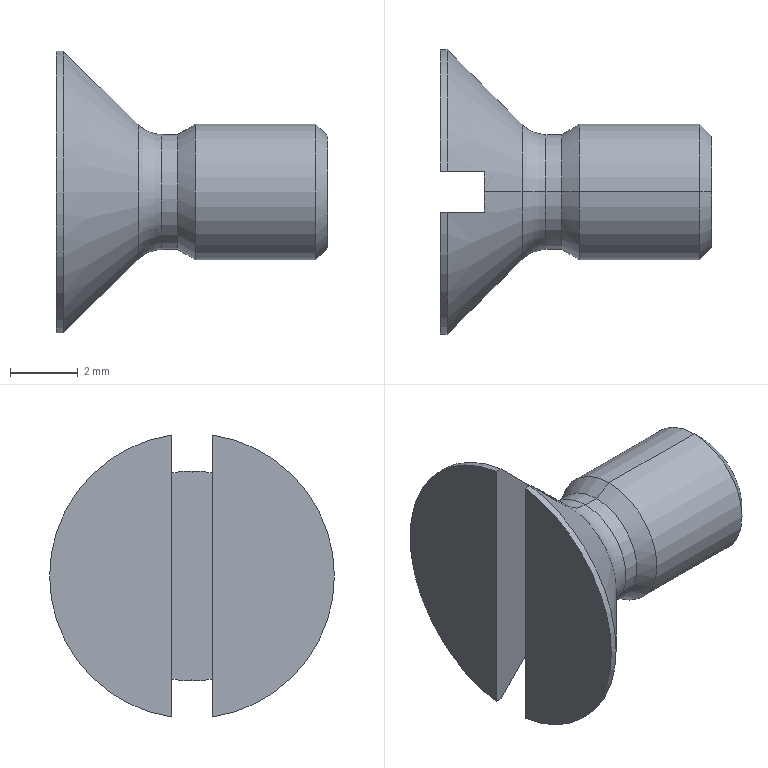Part | SolidWorks | features Chamfer 1, Cut 1, LPattern 1, RevCut 1, Revolution 1 | 1 solid | 20 faces | box 8 x 8.4 x 8.314 mm | volume 133.872 mm3 | cone 6 | cylinder 6 | plane 6 | torus 2 | commonest cylinder face diameters 3.394 x2 4 x2 8.4 x2
STEP:
#1=CARTESIAN_POINT('',(8.,0.,-1.65));
#2=VERTEX_POINT('',#1);
#3=CARTESIAN_POINT('',(8.,0.,1.65));
#4=VERTEX_POINT('',#3);
#5=CARTESIAN_POINT('',(8.,0.,0.));
#6=DIRECTION('',(1.,0.,0.));
#7=DIRECTION('',(0.,0.,1.));
#8=AXIS2_PLACEMENT_3D('',#5,#6,#7);
#9=CIRCLE('',#8,1.65);
#10=EDGE_CURVE('',#2,#4,#9,.T.);
#11=ORIENTED_EDGE('',*,*,#10,.F.);
#12=CARTESIAN_POINT('',(7.65,0.,-2.));
#13=VERTEX_POINT('',#12);
#14=CARTESIAN_POINT('',(7.65,0.,-2.));
#15=DIRECTION('',(-0.7071,0.,-0.7071));
#16=VECTOR('',#15,1000.);
#17=LINE('',#14,#16);
#18=EDGE_CURVE('',#2,#13,#17,.T.);
#19=ORIENTED_EDGE('',*,*,#18,.T.);
#20=CARTESIAN_POINT('',(7.65,0.,2.));
#21=VERTEX_POINT('',#20);
#22=CARTESIAN_POINT('',(7.65,0.,0.));
#23=DIRECTION('',(-1.,0.,0.));
#24=DIRECTION('',(0.,0.,1.));
#25=AXIS2_PLACEMENT_3D('',#22,#23,#24);
#26=CIRCLE('',#25,2.);
#27=EDGE_CURVE('',#21,#13,#26,.T.);
#28=ORIENTED_EDGE('',*,*,#27,.F.);
#29=CARTESIAN_POINT('',(7.65,0.,2.));
#30=DIRECTION('',(-0.7071,0.,0.7071));
#31=VECTOR('',#30,1000.);
#32=LINE('',#29,#31);
#33=EDGE_CURVE('',#4,#21,#32,.T.);
#34=ORIENTED_EDGE('',*,*,#33,.F.);
#35=EDGE_LOOP('',(#11,#19,#28,#34));
#36=FACE_OUTER_BOUND('',#35,.T.);
#37=CARTESIAN_POINT('',(7.65,0.,0.));
#38=DIRECTION('',(-1.,0.,0.));
#39=DIRECTION('',(0.,0.,1.));
#40=AXIS2_PLACEMENT_3D('',#37,#38,#39);
#41=CONICAL_SURFACE('',#40,2.,0.7854);
#42=ADVANCED_FACE('',(#36),#41,.T.);
#43=ORIENTED_EDGE('',*,*,#27,.T.);
#44=CARTESIAN_POINT('',(4.1,0.,-2.));
#45=VERTEX_POINT('',#44);
#46=CARTESIAN_POINT('',(0.,0.,-2.));
#47=DIRECTION('',(-1.,0.,0.));
#48=VECTOR('',#47,1000.);
#49=LINE('',#46,#48);
#50=EDGE_CURVE('',#13,#45,#49,.T.);
#51=ORIENTED_EDGE('',*,*,#50,.T.);
#52=CARTESIAN_POINT('',(4.1,0.,2.));
#53=VERTEX_POINT('',#52);
#54=CARTESIAN_POINT('',(4.1,0.,0.));
#55=DIRECTION('',(-1.,0.,0.));
#56=DIRECTION('',(0.,0.,1.));
#57=AXIS2_PLACEMENT_3D('',#54,#55,#56);
#58=CIRCLE('',#57,2.);
#59=EDGE_CURVE('',#53,#45,#58,.T.);
#60=ORIENTED_EDGE('',*,*,#59,.F.);
#61=CARTESIAN_POINT('',(0.,0.,2.));
#62=DIRECTION('',(-1.,0.,0.));
#63=VECTOR('',#62,1000.);
#64=LINE('',#61,#63);
#65=EDGE_CURVE('',#21,#53,#64,.T.);
#66=ORIENTED_EDGE('',*,*,#65,.F.);
#67=EDGE_LOOP('',(#43,#51,#60,#66));
#68=FACE_OUTER_BOUND('',#67,.T.);
#69=CARTESIAN_POINT('',(0.,0.,0.));
#70=DIRECTION('',(-1.,0.,0.));
#71=DIRECTION('',(0.,0.,1.));
#72=AXIS2_PLACEMENT_3D('',#69,#70,#71);
#73=CYLINDRICAL_SURFACE('',#72,2.);
#74=ADVANCED_FACE('',(#68),#73,.T.);
#75=CARTESIAN_POINT('',(3.575,0.,1.697));
#76=VERTEX_POINT('',#75);
#77=CARTESIAN_POINT('',(3.575,0.,-1.697));
#78=VERTEX_POINT('',#77);
#79=CARTESIAN_POINT('',(3.575,0.,0.));
#80=DIRECTION('',(-1.,0.,0.));
#81=DIRECTION('',(0.,0.,1.));
#82=AXIS2_PLACEMENT_3D('',#79,#80,#81);
#83=CIRCLE('',#82,1.697);
#84=EDGE_CURVE('',#76,#78,#83,.T.);
#85=ORIENTED_EDGE('',*,*,#84,.F.);
#86=CARTESIAN_POINT('',(4.1,0.,2.));
#87=DIRECTION('',(0.866,0.,0.5));
#88=VECTOR('',#87,1000.);
#89=LINE('',#86,#88);
#90=EDGE_CURVE('',#76,#53,#89,.T.);
#91=ORIENTED_EDGE('',*,*,#90,.T.);
#92=ORIENTED_EDGE('',*,*,#59,.T.);
#93=CARTESIAN_POINT('',(4.1,0.,-2.));
#94=DIRECTION('',(0.866,0.,-0.5));
#95=VECTOR('',#94,1000.);
#96=LINE('',#93,#95);
#97=EDGE_CURVE('',#78,#45,#96,.T.);
#98=ORIENTED_EDGE('',*,*,#97,.F.);
#99=EDGE_LOOP('',(#85,#91,#92,#98));
#100=FACE_OUTER_BOUND('',#99,.T.);
#101=CARTESIAN_POINT('',(4.1,0.,0.));
#102=DIRECTION('',(1.,0.,0.));
#103=DIRECTION('',(0.,0.,-1.));
#104=AXIS2_PLACEMENT_3D('',#101,#102,#103);
#105=CONICAL_SURFACE('',#104,2.,0.5236);
#106=ADVANCED_FACE('',(#100),#105,.T.);
#107=ORIENTED_EDGE('',*,*,#84,.T.);
#108=CARTESIAN_POINT('',(3.114,0.,-1.697));
#109=VERTEX_POINT('',#108);
#110=CARTESIAN_POINT('',(0.,0.,-1.697));
#111=DIRECTION('',(-1.,0.,0.));
#112=VECTOR('',#111,1000.);
#113=LINE('',#110,#112);
#114=EDGE_CURVE('',#78,#109,#113,.T.);
#115=ORIENTED_EDGE('',*,*,#114,.T.);
#116=CARTESIAN_POINT('',(3.114,0.,1.697));
#117=VERTEX_POINT('',#116);
#118=CARTESIAN_POINT('',(3.114,0.,0.));
#119=DIRECTION('',(-1.,0.,0.));
#120=DIRECTION('',(0.,0.,1.));
#121=AXIS2_PLACEMENT_3D('',#118,#119,#120);
#122=CIRCLE('',#121,1.697);
#123=EDGE_CURVE('',#117,#109,#122,.T.);
#124=ORIENTED_EDGE('',*,*,#123,.F.);
#125=CARTESIAN_POINT('',(0.,0.,1.697));
#126=DIRECTION('',(-1.,0.,0.));
#127=VECTOR('',#126,1000.);
#128=LINE('',#125,#127);
#129=EDGE_CURVE('',#76,#117,#128,.T.);
#130=ORIENTED_EDGE('',*,*,#129,.F.);
#131=EDGE_LOOP('',(#107,#115,#124,#130));
#132=FACE_OUTER_BOUND('',#131,.T.);
#133=CARTESIAN_POINT('',(0.,0.,0.));
#134=DIRECTION('',(-1.,0.,0.));
#135=DIRECTION('',(0.,0.,1.));
#136=AXIS2_PLACEMENT_3D('',#133,#134,#135);
#137=CYLINDRICAL_SURFACE('',#136,1.697);
#138=ADVANCED_FACE('',(#132),#137,.T.);
#139=CARTESIAN_POINT('',(2.407,0.,-1.99));
#140=VERTEX_POINT('',#139);
#141=CARTESIAN_POINT('',(2.407,0.,1.99));
#142=VERTEX_POINT('',#141);
#143=CARTESIAN_POINT('',(2.407,0.,0.));
#144=DIRECTION('',(-1.,0.,0.));
#145=DIRECTION('',(0.,0.,1.));
#146=AXIS2_PLACEMENT_3D('',#143,#144,#145);
#147=CIRCLE('',#146,1.99);
#148=EDGE_CURVE('',#140,#142,#147,.T.);
#149=ORIENTED_EDGE('',*,*,#148,.F.);
#150=CARTESIAN_POINT('',(3.114,0.,-2.697));
#151=DIRECTION('',(0.,1.,0.));
#152=DIRECTION('',(0.,0.,1.));
#153=AXIS2_PLACEMENT_3D('',#150,#151,#152);
#154=CIRCLE('',#153,1.);
#155=EDGE_CURVE('',#140,#109,#154,.T.);
#156=ORIENTED_EDGE('',*,*,#155,.T.);
#157=CARTESIAN_POINT('',(3.114,0.,0.));
#158=DIRECTION('',(-1.,0.,0.));
#159=DIRECTION('',(0.,0.,1.));
#160=AXIS2_PLACEMENT_3D('',#157,#158,#159);
#161=CIRCLE('',#160,1.697);
#162=EDGE_CURVE('',#109,#117,#161,.T.);
#163=ORIENTED_EDGE('',*,*,#162,.T.);
#164=CARTESIAN_POINT('',(3.114,0.,2.697));
#165=DIRECTION('',(0.,-1.,0.));
#166=DIRECTION('',(0.,0.,-1.));
#167=AXIS2_PLACEMENT_3D('',#164,#165,#166);
#168=CIRCLE('',#167,1.);
#169=EDGE_CURVE('',#142,#117,#168,.T.);
#170=ORIENTED_EDGE('',*,*,#169,.F.);
#171=EDGE_LOOP('',(#149,#156,#163,#170));
#172=FACE_OUTER_BOUND('',#171,.T.);
#173=CARTESIAN_POINT('',(3.114,0.,0.));
#174=DIRECTION('',(-1.,0.,0.));
#175=DIRECTION('',(0.,0.,1.));
#176=AXIS2_PLACEMENT_3D('',#173,#174,#175);
#177=TOROIDAL_SURFACE('',#176,2.697,1.);
#178=ADVANCED_FACE('',(#172),#177,.F.);
#179=CARTESIAN_POINT('',(2.407,0.,0.));
#180=DIRECTION('',(-1.,0.,0.));
#181=DIRECTION('',(0.,0.,1.));
#182=AXIS2_PLACEMENT_3D('',#179,#180,#181);
#183=CIRCLE('',#182,1.99);
#184=EDGE_CURVE('',#142,#140,#183,.T.);
#185=ORIENTED_EDGE('',*,*,#184,.T.);
#186=CARTESIAN_POINT('',(1.3,0.,-3.097));
#187=VERTEX_POINT('',#186);
#188=CARTESIAN_POINT('',(2.407,0.,-1.99));
#189=DIRECTION('',(-0.7071,0.,-0.7071));
#190=VECTOR('',#189,1000.);
#191=LINE('',#188,#190);
#192=EDGE_CURVE('',#140,#187,#191,.T.);
#193=ORIENTED_EDGE('',*,*,#192,.T.);
#194=CARTESIAN_POINT('',(1.3,0.6,-3.038));
#195=VERTEX_POINT('',#194);
#196=CARTESIAN_POINT('',(1.3,0.,0.));
#197=DIRECTION('',(-1.,0.,0.));
#198=DIRECTION('',(0.,0.,1.));
#199=AXIS2_PLACEMENT_3D('',#196,#197,#198);
#200=CIRCLE('',#199,3.097);
#201=EDGE_CURVE('',#195,#187,#200,.T.);
#202=ORIENTED_EDGE('',*,*,#201,.F.);
#203=CARTESIAN_POINT('',(0.1969,0.6,-4.157));
#204=VERTEX_POINT('',#203);
#205=CARTESIAN_POINT('',(1.3,0.6,-3.038));
#206=CARTESIAN_POINT('',(0.9332,0.6,-3.412));
#207=CARTESIAN_POINT('',(0.5653,0.6,-3.785));
#208=CARTESIAN_POINT('',(0.1969,0.6,-4.157));
#209=B_SPLINE_CURVE_WITH_KNOTS('',3,(#205,#206,#207,#208),.UNSPECIFIED.,.F.,.F.,(4,4),(0.01666,0.01824),.UNSPECIFIED.);
#210=EDGE_CURVE('',#195,#204,#209,.T.);
#211=ORIENTED_EDGE('',*,*,#210,.T.);
#212=CARTESIAN_POINT('',(0.1969,0.6,4.157));
#213=VERTEX_POINT('',#212);
#214=CARTESIAN_POINT('',(0.1969,0.,0.));
#215=DIRECTION('',(-1.,0.,0.));
#216=DIRECTION('',(0.,0.,1.));
#217=AXIS2_PLACEMENT_3D('',#214,#215,#216);
#218=CIRCLE('',#217,4.2);
#219=EDGE_CURVE('',#213,#204,#218,.T.);
#220=ORIENTED_EDGE('',*,*,#219,.F.);
#221=CARTESIAN_POINT('',(1.3,0.6,3.038));
#222=VERTEX_POINT('',#221);
#223=CARTESIAN_POINT('',(0.1969,0.6,4.157));
#224=CARTESIAN_POINT('',(0.5653,0.6,3.785));
#225=CARTESIAN_POINT('',(0.9332,0.6,3.412));
#226=CARTESIAN_POINT('',(1.3,0.6,3.038));
#227=B_SPLINE_CURVE_WITH_KNOTS('',3,(#223,#224,#225,#226),.UNSPECIFIED.,.F.,.F.,(4,4),(0.0071,0.008671),.UNSPECIFIED.);
#228=EDGE_CURVE('',#213,#222,#227,.T.);
#229=ORIENTED_EDGE('',*,*,#228,.T.);
#230=CARTESIAN_POINT('',(1.3,0.,3.097));
#231=VERTEX_POINT('',#230);
#232=CARTESIAN_POINT('',(1.3,0.,0.));
#233=DIRECTION('',(-1.,0.,0.));
#234=DIRECTION('',(0.,0.,1.));
#235=AXIS2_PLACEMENT_3D('',#232,#233,#234);
#236=CIRCLE('',#235,3.097);
#237=EDGE_CURVE('',#231,#222,#236,.T.);
#238=ORIENTED_EDGE('',*,*,#237,.F.);
#239=CARTESIAN_POINT('',(2.407,0.,1.99));
#240=DIRECTION('',(-0.7071,0.,0.7071));
#241=VECTOR('',#240,1000.);
#242=LINE('',#239,#241);
#243=EDGE_CURVE('',#142,#231,#242,.T.);
#244=ORIENTED_EDGE('',*,*,#243,.F.);
#245=EDGE_LOOP('',(#185,#193,#202,#211,#220,#229,#238,#244));
#246=FACE_OUTER_BOUND('',#245,.T.);
#247=CARTESIAN_POINT('',(2.407,0.,0.));
#248=DIRECTION('',(-1.,0.,0.));
#249=DIRECTION('',(0.,0.,1.));
#250=AXIS2_PLACEMENT_3D('',#247,#248,#249);
#251=CONICAL_SURFACE('',#250,1.99,0.7854);
#252=ADVANCED_FACE('',(#246),#251,.T.);
#253=CARTESIAN_POINT('',(0.,0.6,4.157));
#254=VERTEX_POINT('',#253);
#255=CARTESIAN_POINT('',(0.,0.6,-4.157));
#256=VERTEX_POINT('',#255);
#257=CARTESIAN_POINT('',(0.,0.,0.));
#258=DIRECTION('',(-1.,0.,0.));
#259=DIRECTION('',(0.,0.,1.));
#260=AXIS2_PLACEMENT_3D('',#257,#258,#259);
#261=CIRCLE('',#260,4.2);
#262=EDGE_CURVE('',#254,#256,#261,.T.);
#263=ORIENTED_EDGE('',*,*,#262,.T.);
#264=CARTESIAN_POINT('',(0.,0.6,-4.157));
#265=DIRECTION('',(0.,0.,-1.));
#266=VECTOR('',#265,1000.);
#267=LINE('',#264,#266);
#268=EDGE_CURVE('',#254,#256,#267,.T.);
#269=ORIENTED_EDGE('',*,*,#268,.F.);
#270=EDGE_LOOP('',(#263,#269));
#271=FACE_OUTER_BOUND('',#270,.T.);
#272=CARTESIAN_POINT('',(0.,0.,0.));
#273=DIRECTION('',(1.,0.,0.));
#274=DIRECTION('',(0.,0.,-1.));
#275=AXIS2_PLACEMENT_3D('',#272,#273,#274);
#276=PLANE('',#275);
#277=ADVANCED_FACE('',(#271),#276,.F.);
#278=ORIENTED_EDGE('',*,*,#219,.T.);
#279=CARTESIAN_POINT('',(1.3,0.6,-4.157));
#280=DIRECTION('',(-1.,0.,0.));
#281=VECTOR('',#280,1000.);
#282=LINE('',#279,#281);
#283=EDGE_CURVE('',#204,#256,#282,.T.);
#284=ORIENTED_EDGE('',*,*,#283,.T.);
#285=ORIENTED_EDGE('',*,*,#262,.F.);
#286=CARTESIAN_POINT('',(1.3,0.6,4.157));
#287=DIRECTION('',(-1.,0.,0.));
#288=VECTOR('',#287,1000.);
#289=LINE('',#286,#288);
#290=EDGE_CURVE('',#213,#254,#289,.T.);
#291=ORIENTED_EDGE('',*,*,#290,.F.);
#292=EDGE_LOOP('',(#278,#284,#285,#291));
#293=FACE_OUTER_BOUND('',#292,.T.);
#294=CARTESIAN_POINT('',(0.,0.,0.));
#295=DIRECTION('',(-1.,0.,0.));
#296=DIRECTION('',(0.,0.,1.));
#297=AXIS2_PLACEMENT_3D('',#294,#295,#296);
#298=CYLINDRICAL_SURFACE('',#297,4.2);
#299=ADVANCED_FACE('',(#293),#298,.T.);
#300=CARTESIAN_POINT('',(0.,-0.6,-4.157));
#301=VERTEX_POINT('',#300);
#302=CARTESIAN_POINT('',(0.,-0.6,4.157));
#303=VERTEX_POINT('',#302);
#304=CARTESIAN_POINT('',(0.,0.,0.));
#305=DIRECTION('',(-1.,0.,0.));
#306=DIRECTION('',(0.,0.,1.));
#307=AXIS2_PLACEMENT_3D('',#304,#305,#306);
#308=CIRCLE('',#307,4.2);
#309=EDGE_CURVE('',#301,#303,#308,.T.);
#310=ORIENTED_EDGE('',*,*,#309,.T.);
#311=CARTESIAN_POINT('',(0.,-0.6,-4.157));
#312=DIRECTION('',(0.,0.,1.));
#313=VECTOR('',#312,1000.);
#314=LINE('',#311,#313);
#315=EDGE_CURVE('',#301,#303,#314,.T.);
#316=ORIENTED_EDGE('',*,*,#315,.F.);
#317=EDGE_LOOP('',(#310,#316));
#318=FACE_OUTER_BOUND('',#317,.T.);
#319=CARTESIAN_POINT('',(0.,0.,0.));
#320=DIRECTION('',(1.,0.,0.));
#321=DIRECTION('',(0.,0.,-1.));
#322=AXIS2_PLACEMENT_3D('',#319,#320,#321);
#323=PLANE('',#322);
#324=ADVANCED_FACE('',(#318),#323,.F.);
#325=CARTESIAN_POINT('',(0.1969,-0.6,-4.157));
#326=VERTEX_POINT('',#325);
#327=CARTESIAN_POINT('',(0.1969,-0.6,4.157));
#328=VERTEX_POINT('',#327);
#329=CARTESIAN_POINT('',(0.1969,0.,0.));
#330=DIRECTION('',(-1.,0.,0.));
#331=DIRECTION('',(0.,0.,1.));
#332=AXIS2_PLACEMENT_3D('',#329,#330,#331);
#333=CIRCLE('',#332,4.2);
#334=EDGE_CURVE('',#326,#328,#333,.T.);
#335=ORIENTED_EDGE('',*,*,#334,.T.);
#336=CARTESIAN_POINT('',(1.3,-0.6,4.157));
#337=DIRECTION('',(-1.,0.,0.));
#338=VECTOR('',#337,1000.);
#339=LINE('',#336,#338);
#340=EDGE_CURVE('',#328,#303,#339,.T.);
#341=ORIENTED_EDGE('',*,*,#340,.T.);
#342=ORIENTED_EDGE('',*,*,#309,.F.);
#343=CARTESIAN_POINT('',(1.3,-0.6,-4.157));
#344=DIRECTION('',(-1.,0.,0.));
#345=VECTOR('',#344,1000.);
#346=LINE('',#343,#345);
#347=EDGE_CURVE('',#326,#301,#346,.T.);
#348=ORIENTED_EDGE('',*,*,#347,.F.);
#349=EDGE_LOOP('',(#335,#341,#342,#348));
#350=FACE_OUTER_BOUND('',#349,.T.);
#351=CARTESIAN_POINT('',(0.,0.,0.));
#352=DIRECTION('',(-1.,0.,0.));
#353=DIRECTION('',(0.,0.,1.));
#354=AXIS2_PLACEMENT_3D('',#351,#352,#353);
#355=CYLINDRICAL_SURFACE('',#354,4.2);
#356=ADVANCED_FACE('',(#350),#355,.T.);
#357=ORIENTED_EDGE('',*,*,#192,.F.);
#358=ORIENTED_EDGE('',*,*,#148,.T.);
#359=ORIENTED_EDGE('',*,*,#243,.T.);
#360=CARTESIAN_POINT('',(1.3,-0.6,3.038));
#361=VERTEX_POINT('',#360);
#362=CARTESIAN_POINT('',(1.3,0.,0.));
#363=DIRECTION('',(-1.,0.,0.));
#364=DIRECTION('',(0.,0.,1.));
#365=AXIS2_PLACEMENT_3D('',#362,#363,#364);
#366=CIRCLE('',#365,3.097);
#367=EDGE_CURVE('',#361,#231,#366,.T.);
#368=ORIENTED_EDGE('',*,*,#367,.F.);
#369=CARTESIAN_POINT('',(1.3,-0.6,3.038));
#370=CARTESIAN_POINT('',(0.9332,-0.6,3.412));
#371=CARTESIAN_POINT('',(0.5653,-0.6,3.785));
#372=CARTESIAN_POINT('',(0.1969,-0.6,4.157));
#373=B_SPLINE_CURVE_WITH_KNOTS('',3,(#369,#370,#371,#372),.UNSPECIFIED.,.F.,.F.,(4,4),(0.01666,0.01824),.UNSPECIFIED.);
#374=EDGE_CURVE('',#361,#328,#373,.T.);
#375=ORIENTED_EDGE('',*,*,#374,.T.);
#376=ORIENTED_EDGE('',*,*,#334,.F.);
#377=CARTESIAN_POINT('',(1.3,-0.6,-3.038));
#378=VERTEX_POINT('',#377);
#379=CARTESIAN_POINT('',(0.1969,-0.6,-4.157));
#380=CARTESIAN_POINT('',(0.5653,-0.6,-3.785));
#381=CARTESIAN_POINT('',(0.9332,-0.6,-3.412));
#382=CARTESIAN_POINT('',(1.3,-0.6,-3.038));
#383=B_SPLINE_CURVE_WITH_KNOTS('',3,(#379,#380,#381,#382),.UNSPECIFIED.,.F.,.F.,(4,4),(0.0071,0.008671),.UNSPECIFIED.);
#384=EDGE_CURVE('',#326,#378,#383,.T.);
#385=ORIENTED_EDGE('',*,*,#384,.T.);
#386=CARTESIAN_POINT('',(1.3,0.,0.));
#387=DIRECTION('',(-1.,0.,0.));
#388=DIRECTION('',(0.,0.,1.));
#389=AXIS2_PLACEMENT_3D('',#386,#387,#388);
#390=CIRCLE('',#389,3.097);
#391=EDGE_CURVE('',#187,#378,#390,.T.);
#392=ORIENTED_EDGE('',*,*,#391,.F.);
#393=EDGE_LOOP('',(#357,#358,#359,#368,#375,#376,#385,#392));
#394=FACE_OUTER_BOUND('',#393,.T.);
#395=CARTESIAN_POINT('',(2.407,0.,0.));
#396=DIRECTION('',(-1.,0.,0.));
#397=DIRECTION('',(0.,0.,1.));
#398=AXIS2_PLACEMENT_3D('',#395,#396,#397);
#399=CONICAL_SURFACE('',#398,1.99,0.7854);
#400=ADVANCED_FACE('',(#394),#399,.T.);
#401=ORIENTED_EDGE('',*,*,#155,.F.);
#402=ORIENTED_EDGE('',*,*,#184,.F.);
#403=ORIENTED_EDGE('',*,*,#169,.T.);
#404=ORIENTED_EDGE('',*,*,#123,.T.);
#405=EDGE_LOOP('',(#401,#402,#403,#404));
#406=FACE_OUTER_BOUND('',#405,.T.);
#407=CARTESIAN_POINT('',(3.114,0.,0.));
#408=DIRECTION('',(-1.,0.,0.));
#409=DIRECTION('',(0.,0.,1.));
#410=AXIS2_PLACEMENT_3D('',#407,#408,#409);
#411=TOROIDAL_SURFACE('',#410,2.697,1.);
#412=ADVANCED_FACE('',(#406),#411,.F.);
#413=ORIENTED_EDGE('',*,*,#114,.F.);
#414=CARTESIAN_POINT('',(3.575,0.,0.));
#415=DIRECTION('',(-1.,0.,0.));
#416=DIRECTION('',(0.,0.,1.));
#417=AXIS2_PLACEMENT_3D('',#414,#415,#416);
#418=CIRCLE('',#417,1.697);
#419=EDGE_CURVE('',#78,#76,#418,.T.);
#420=ORIENTED_EDGE('',*,*,#419,.T.);
#421=ORIENTED_EDGE('',*,*,#129,.T.);
#422=ORIENTED_EDGE('',*,*,#162,.F.);
#423=EDGE_LOOP('',(#413,#420,#421,#422));
#424=FACE_OUTER_BOUND('',#423,.T.);
#425=CARTESIAN_POINT('',(0.,0.,0.));
#426=DIRECTION('',(-1.,0.,0.));
#427=DIRECTION('',(0.,0.,1.));
#428=AXIS2_PLACEMENT_3D('',#425,#426,#427);
#429=CYLINDRICAL_SURFACE('',#428,1.697);
#430=ADVANCED_FACE('',(#424),#429,.T.);
#431=ORIENTED_EDGE('',*,*,#90,.F.);
#432=ORIENTED_EDGE('',*,*,#419,.F.);
#433=ORIENTED_EDGE('',*,*,#97,.T.);
#434=CARTESIAN_POINT('',(4.1,0.,0.));
#435=DIRECTION('',(-1.,0.,0.));
#436=DIRECTION('',(0.,0.,1.));
#437=AXIS2_PLACEMENT_3D('',#434,#435,#436);
#438=CIRCLE('',#437,2.);
#439=EDGE_CURVE('',#45,#53,#438,.T.);
#440=ORIENTED_EDGE('',*,*,#439,.T.);
#441=EDGE_LOOP('',(#431,#432,#433,#440));
#442=FACE_OUTER_BOUND('',#441,.T.);
#443=CARTESIAN_POINT('',(4.1,0.,0.));
#444=DIRECTION('',(1.,0.,0.));
#445=DIRECTION('',(0.,0.,-1.));
#446=AXIS2_PLACEMENT_3D('',#443,#444,#445);
#447=CONICAL_SURFACE('',#446,2.,0.5236);
#448=ADVANCED_FACE('',(#442),#447,.T.);
#449=ORIENTED_EDGE('',*,*,#50,.F.);
#450=CARTESIAN_POINT('',(7.65,0.,0.));
#451=DIRECTION('',(-1.,0.,0.));
#452=DIRECTION('',(0.,0.,1.));
#453=AXIS2_PLACEMENT_3D('',#450,#451,#452);
#454=CIRCLE('',#453,2.);
#455=EDGE_CURVE('',#13,#21,#454,.T.);
#456=ORIENTED_EDGE('',*,*,#455,.T.);
#457=ORIENTED_EDGE('',*,*,#65,.T.);
#458=ORIENTED_EDGE('',*,*,#439,.F.);
#459=EDGE_LOOP('',(#449,#456,#457,#458));
#460=FACE_OUTER_BOUND('',#459,.T.);
#461=CARTESIAN_POINT('',(0.,0.,0.));
#462=DIRECTION('',(-1.,0.,0.));
#463=DIRECTION('',(0.,0.,1.));
#464=AXIS2_PLACEMENT_3D('',#461,#462,#463);
#465=CYLINDRICAL_SURFACE('',#464,2.);
#466=ADVANCED_FACE('',(#460),#465,.T.);
#467=CARTESIAN_POINT('',(8.,0.,0.));
#468=DIRECTION('',(1.,0.,0.));
#469=DIRECTION('',(0.,0.,1.));
#470=AXIS2_PLACEMENT_3D('',#467,#468,#469);
#471=CIRCLE('',#470,1.65);
#472=EDGE_CURVE('',#4,#2,#471,.T.);
#473=ORIENTED_EDGE('',*,*,#472,.T.);
#474=ORIENTED_EDGE('',*,*,#10,.T.);
#475=EDGE_LOOP('',(#473,#474));
#476=FACE_OUTER_BOUND('',#475,.T.);
#477=CARTESIAN_POINT('',(8.,2.,0.));
#478=DIRECTION('',(-1.,0.,0.));
#479=DIRECTION('',(0.,0.,1.));
#480=AXIS2_PLACEMENT_3D('',#477,#478,#479);
#481=PLANE('',#480);
#482=ADVANCED_FACE('',(#476),#481,.F.);
#483=ORIENTED_EDGE('',*,*,#18,.F.);
#484=ORIENTED_EDGE('',*,*,#472,.F.);
#485=ORIENTED_EDGE('',*,*,#33,.T.);
#486=ORIENTED_EDGE('',*,*,#455,.F.);
#487=EDGE_LOOP('',(#483,#484,#485,#486));
#488=FACE_OUTER_BOUND('',#487,.T.);
#489=CARTESIAN_POINT('',(7.65,0.,0.));
#490=DIRECTION('',(-1.,0.,0.));
#491=DIRECTION('',(0.,0.,1.));
#492=AXIS2_PLACEMENT_3D('',#489,#490,#491);
#493=CONICAL_SURFACE('',#492,2.,0.7854);
#494=ADVANCED_FACE('',(#488),#493,.T.);
#495=ORIENTED_EDGE('',*,*,#290,.T.);
#496=ORIENTED_EDGE('',*,*,#268,.T.);
#497=ORIENTED_EDGE('',*,*,#283,.F.);
#498=ORIENTED_EDGE('',*,*,#210,.F.);
#499=CARTESIAN_POINT('',(1.3,0.6,-4.157));
#500=DIRECTION('',(0.,0.,-1.));
#501=VECTOR('',#500,1000.);
#502=LINE('',#499,#501);
#503=EDGE_CURVE('',#222,#195,#502,.T.);
#504=ORIENTED_EDGE('',*,*,#503,.F.);
#505=ORIENTED_EDGE('',*,*,#228,.F.);
#506=EDGE_LOOP('',(#495,#496,#497,#498,#504,#505));
#507=FACE_OUTER_BOUND('',#506,.T.);
#508=CARTESIAN_POINT('',(1.3,0.6,-4.157));
#509=DIRECTION('',(0.,1.,0.));
#510=DIRECTION('',(0.,0.,1.));
#511=AXIS2_PLACEMENT_3D('',#508,#509,#510);
#512=PLANE('',#511);
#513=ADVANCED_FACE('',(#507),#512,.F.);
#514=ORIENTED_EDGE('',*,*,#347,.T.);
#515=ORIENTED_EDGE('',*,*,#315,.T.);
#516=ORIENTED_EDGE('',*,*,#340,.F.);
#517=ORIENTED_EDGE('',*,*,#374,.F.);
#518=CARTESIAN_POINT('',(1.3,-0.6,-4.157));
#519=DIRECTION('',(0.,0.,1.));
#520=VECTOR('',#519,1000.);
#521=LINE('',#518,#520);
#522=EDGE_CURVE('',#378,#361,#521,.T.);
#523=ORIENTED_EDGE('',*,*,#522,.F.);
#524=ORIENTED_EDGE('',*,*,#384,.F.);
#525=EDGE_LOOP('',(#514,#515,#516,#517,#523,#524));
#526=FACE_OUTER_BOUND('',#525,.T.);
#527=CARTESIAN_POINT('',(1.3,-0.6,-4.157));
#528=DIRECTION('',(0.,-1.,0.));
#529=DIRECTION('',(0.,0.,-1.));
#530=AXIS2_PLACEMENT_3D('',#527,#528,#529);
#531=PLANE('',#530);
#532=ADVANCED_FACE('',(#526),#531,.F.);
#533=ORIENTED_EDGE('',*,*,#201,.T.);
#534=ORIENTED_EDGE('',*,*,#391,.T.);
#535=ORIENTED_EDGE('',*,*,#522,.T.);
#536=ORIENTED_EDGE('',*,*,#367,.T.);
#537=ORIENTED_EDGE('',*,*,#237,.T.);
#538=ORIENTED_EDGE('',*,*,#503,.T.);
#539=EDGE_LOOP('',(#533,#534,#535,#536,#537,#538));
#540=FACE_OUTER_BOUND('',#539,.T.);
#541=CARTESIAN_POINT('',(1.3,0.,0.));
#542=DIRECTION('',(-1.,0.,0.));
#543=DIRECTION('',(0.,0.,1.));
#544=AXIS2_PLACEMENT_3D('',#541,#542,#543);
#545=PLANE('',#544);
#546=ADVANCED_FACE('',(#540),#545,.T.);
#547=CLOSED_SHELL('',(#42,#74,#106,#138,#178,#252,#277,#299,#324,#356,#400,#412,#430,#448,#466,#482,#494,#513,#532,#546));
#548=MANIFOLD_SOLID_BREP('',#547);
#549=CARTESIAN_POINT('',(0.,0.,0.));
#550=DIRECTION('',(0.,0.,1.));
#551=DIRECTION('',(1.,0.,0.));
#552=AXIS2_PLACEMENT_3D('',#549,#550,#551);
#553=(LENGTH_UNIT()NAMED_UNIT(*)SI_UNIT(.MILLI.,.METRE.));
#554=UNCERTAINTY_MEASURE_WITH_UNIT(LENGTH_MEASURE(0.00001),#553,'','');
#555=(NAMED_UNIT(*)PLANE_ANGLE_UNIT()SI_UNIT($,.RADIAN.));
#556=(NAMED_UNIT(*)SI_UNIT($,.STERADIAN.)SOLID_ANGLE_UNIT());
#557=(GEOMETRIC_REPRESENTATION_CONTEXT(3)GLOBAL_UNCERTAINTY_ASSIGNED_CONTEXT((#554))GLOBAL_UNIT_ASSIGNED_CONTEXT((#553,#555,#556))REPRESENTATION_CONTEXT('',''));
#558=ADVANCED_BREP_SHAPE_REPRESENTATION('',(#548,#552),#557);